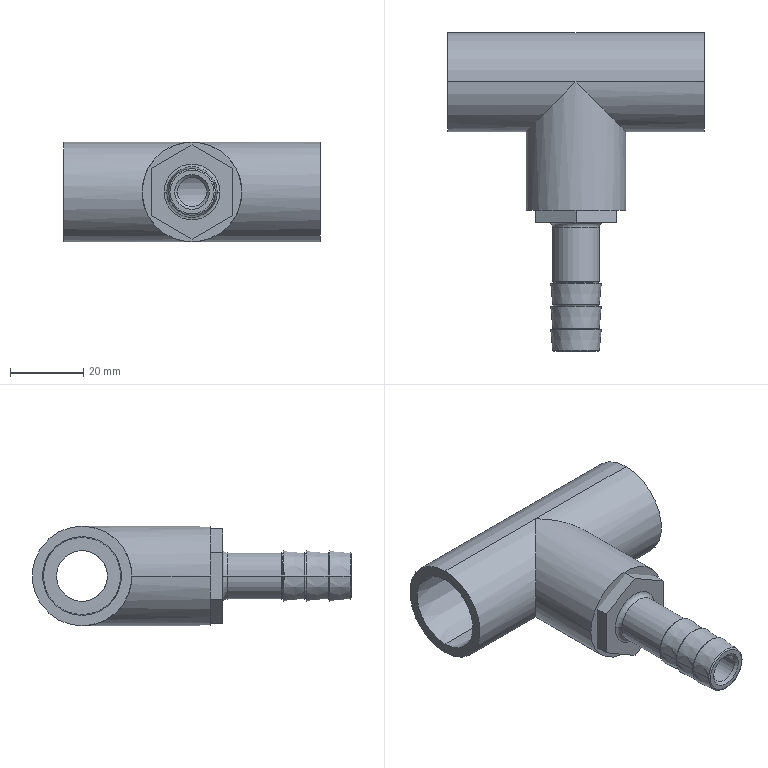Part | SolidWorks | 2 solids | 123 faces | box 69.85 x 87.046 x 27.178 mm | volume 35204 mm3 | cone 67 | plane 19 | torus 16 | cylinder 15 | spline 6 | commonest cylinder face diameters 27.178 x5 12.7 x4 7.95 x2 12.484 x2 13.868 x2